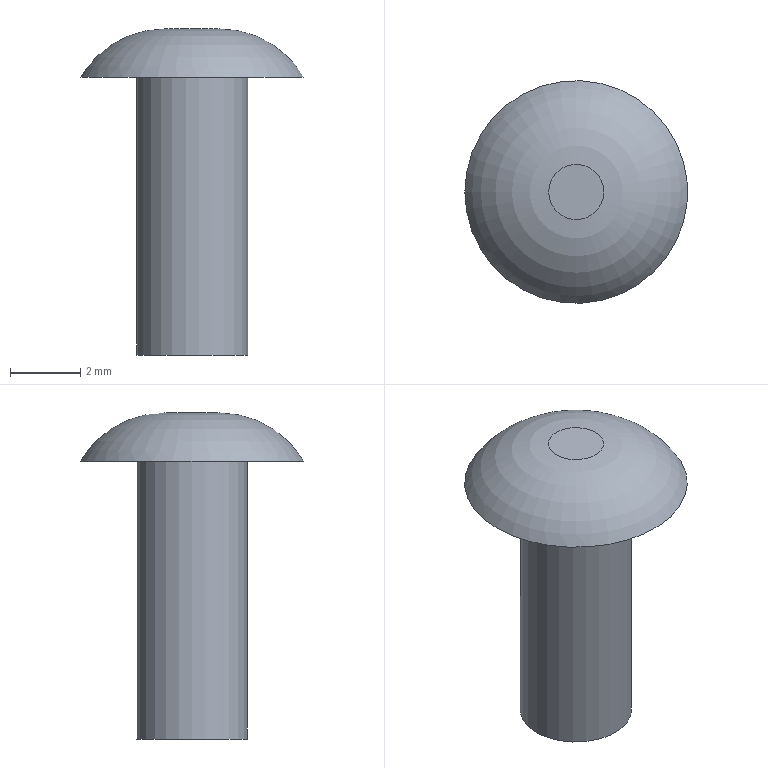Part | NX | features solid 2 | 1 solid | 5 faces | box 6.35 x 6.35 x 9.296 mm | volume 90.532 mm3 | plane 3 | cylinder 1 | torus 1 | commonest cylinder face diameters 3.175 x1
STEP:
#1=CARTESIAN_POINT('',(-0.7874,0.,9.296));
#2=VERTEX_POINT('',#1);
#3=CARTESIAN_POINT('',(0.,0.,9.296));
#4=DIRECTION('',(0.,0.,-1.));
#5=DIRECTION('',(-1.,0.,0.));
#6=AXIS2_PLACEMENT_3D('',#3,#4,#5);
#7=CIRCLE('',#6,0.7874);
#8=EDGE_CURVE('',#2,#2,#7,.T.);
#9=ORIENTED_EDGE('',*,*,#8,.F.);
#10=EDGE_LOOP('',(#9));
#11=FACE_BOUND('',#10,.T.);
#12=CARTESIAN_POINT('',(0.7874,0.,9.296));
#13=DIRECTION('',(0.,0.,1.));
#14=DIRECTION('',(1.,0.,0.));
#15=AXIS2_PLACEMENT_3D('',#12,#13,#14);
#16=PLANE('',#15);
#17=ADVANCED_FACE('',(#11),#16,.T.);
#18=CARTESIAN_POINT('',(-1.587,0.,0.));
#19=VERTEX_POINT('',#18);
#20=CARTESIAN_POINT('',(0.,0.,0.));
#21=DIRECTION('',(0.,0.,-1.));
#22=DIRECTION('',(-1.,0.,0.));
#23=AXIS2_PLACEMENT_3D('',#20,#21,#22);
#24=CIRCLE('',#23,1.587);
#25=EDGE_CURVE('',#19,#19,#24,.T.);
#26=ORIENTED_EDGE('',*,*,#25,.T.);
#27=EDGE_LOOP('',(#26));
#28=FACE_BOUND('',#27,.T.);
#29=CARTESIAN_POINT('',(0.,0.,0.));
#30=DIRECTION('',(0.,0.,-1.));
#31=DIRECTION('',(-1.,0.,0.));
#32=AXIS2_PLACEMENT_3D('',#29,#30,#31);
#33=PLANE('',#32);
#34=ADVANCED_FACE('',(#28),#33,.T.);
#35=CARTESIAN_POINT('',(-1.587,0.,7.925));
#36=VERTEX_POINT('',#35);
#37=CARTESIAN_POINT('',(0.,0.,7.925));
#38=DIRECTION('',(0.,0.,-1.));
#39=DIRECTION('',(-1.,0.,0.));
#40=AXIS2_PLACEMENT_3D('',#37,#38,#39);
#41=CIRCLE('',#40,1.587);
#42=EDGE_CURVE('',#36,#36,#41,.T.);
#43=ORIENTED_EDGE('',*,*,#42,.T.);
#44=EDGE_LOOP('',(#43));
#45=FACE_BOUND('',#44,.T.);
#46=ORIENTED_EDGE('',*,*,#25,.F.);
#47=EDGE_LOOP('',(#46));
#48=FACE_BOUND('',#47,.T.);
#49=CARTESIAN_POINT('',(0.,0.,0.));
#50=DIRECTION('',(0.,0.,-1.));
#51=DIRECTION('',(-1.,0.,0.));
#52=AXIS2_PLACEMENT_3D('',#49,#50,#51);
#53=CYLINDRICAL_SURFACE('',#52,1.587);
#54=ADVANCED_FACE('',(#45,#48),#53,.T.);
#55=CARTESIAN_POINT('',(-3.175,0.,7.925));
#56=VERTEX_POINT('',#55);
#57=CARTESIAN_POINT('',(0.,0.,7.925));
#58=DIRECTION('',(0.,0.,-1.));
#59=DIRECTION('',(-1.,0.,0.));
#60=AXIS2_PLACEMENT_3D('',#57,#58,#59);
#61=CIRCLE('',#60,3.175);
#62=EDGE_CURVE('',#56,#56,#61,.T.);
#63=ORIENTED_EDGE('',*,*,#62,.T.);
#64=EDGE_LOOP('',(#63));
#65=FACE_BOUND('',#64,.T.);
#66=ORIENTED_EDGE('',*,*,#42,.F.);
#67=EDGE_LOOP('',(#66));
#68=FACE_BOUND('',#67,.T.);
#69=CARTESIAN_POINT('',(1.587,0.,7.925));
#70=DIRECTION('',(0.,0.,-1.));
#71=DIRECTION('',(-1.,0.,0.));
#72=AXIS2_PLACEMENT_3D('',#69,#70,#71);
#73=PLANE('',#72);
#74=ADVANCED_FACE('',(#65,#68),#73,.T.);
#75=ORIENTED_EDGE('',*,*,#8,.T.);
#76=EDGE_LOOP('',(#75));
#77=FACE_BOUND('',#76,.T.);
#78=ORIENTED_EDGE('',*,*,#62,.F.);
#79=EDGE_LOOP('',(#78));
#80=FACE_BOUND('',#79,.T.);
#81=CARTESIAN_POINT('',(0.,0.,6.533));
#82=DIRECTION('',(0.,0.,-1.));
#83=DIRECTION('',(-1.,0.,0.));
#84=AXIS2_PLACEMENT_3D('',#81,#82,#83);
#85=DEGENERATE_TOROIDAL_SURFACE('',#84,0.7874,2.764,.T.);
#86=ADVANCED_FACE('',(#77,#80),#85,.T.);
#87=CLOSED_SHELL('',(#17,#34,#54,#74,#86));
#88=MANIFOLD_SOLID_BREP('',#87);
#89=(LENGTH_UNIT()NAMED_UNIT(*)SI_UNIT(.MILLI.,.METRE.));
#90=UNCERTAINTY_MEASURE_WITH_UNIT(LENGTH_MEASURE(0.00001),#89,'','');
#91=(NAMED_UNIT(*)PLANE_ANGLE_UNIT()SI_UNIT($,.RADIAN.));
#92=(NAMED_UNIT(*)SI_UNIT($,.STERADIAN.)SOLID_ANGLE_UNIT());
#93=(GEOMETRIC_REPRESENTATION_CONTEXT(3)GLOBAL_UNCERTAINTY_ASSIGNED_CONTEXT((#90))GLOBAL_UNIT_ASSIGNED_CONTEXT((#89,#91,#92))REPRESENTATION_CONTEXT('',''));
#94=ADVANCED_BREP_SHAPE_REPRESENTATION('',(#88),#93);